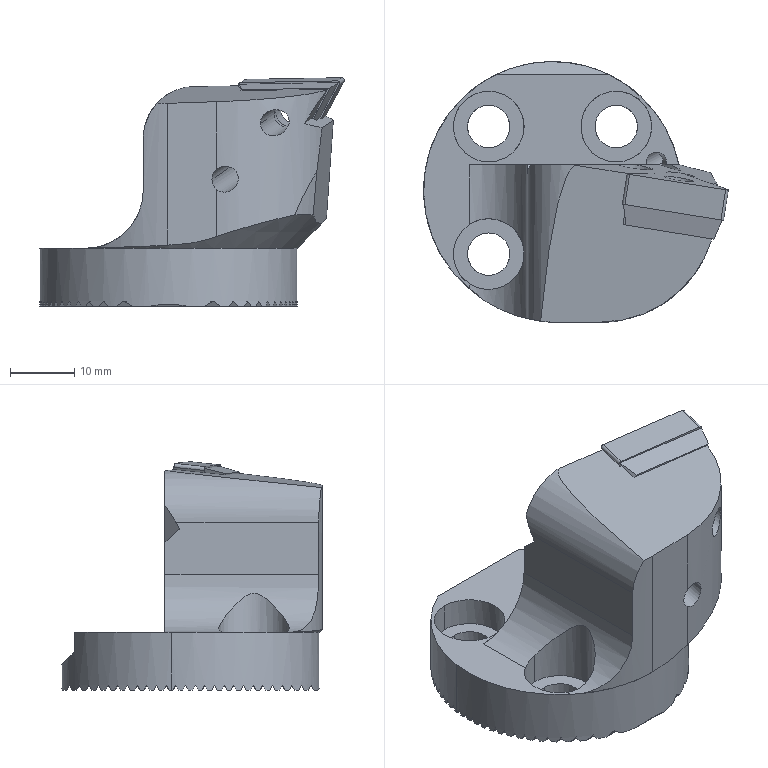NC program | Mastercam | posted with a generic post
Lines 243 to 895 of 11065:
(12 FEMR |TOOL - 4|DIA. OFF. - 4|LEN. - 4|TOOL DIA. - 12.)
N536 T4 M6
N538 G0 G54 G90 X36.247 Y-2.28 C0. B0. S3500 M3
N540 G43 H4 Z84.239 M8
N542 Z36.239
N544 G1 Z8.489 F2000.
N546 X34.611 Y-1.757 Z8.338 F2500.
N548 G3 X33.789 Y-1.629 Z8.265 I-.822 J-2.572
N550 X33.497 Y-1.645 Z8.239 J-2.7
N552 G1 X32.902 Y-1.71
N554 X32.852 Y-1.819
N556 G3 X32.449 Y-4.11 I31.093 J-6.656
N558 G2 X30.953 Y-10.357 I-38.311 J5.87
N560 X-.001 Y-32.641 I-30.954 J10.357
N562 X-6.571 Y-31.973 J32.641
N564 X-17.793 Y-27.363 I6.574 J31.969
N566 G1 X-18.064 Y-27.656
N568 X-18.335 Y-27.949
N570 G3 X-18.91 Y-28.91 Z8.314 I1.979 J-1.836
N572 G1 X-19.466 Y-30.534 Z8.428
N574 G3 X-19.604 Y-31.36 Z8.483 I2.412 J-.826
N576 X-19.603 Y-31.444 Z8.489 I2.55
N578 X-17.107 Y-33.91 I2.549 J.084
N580 G1 X-.868 Y-34.244 F9500.
N582 G3 X-.127 Y-34.252 I.741 J35.984
N584 X31.322 Y-15.762 J35.992
N586 G1 X37.454 Y-4.742
N588 G3 X37.66 Y-3.946 I-1.431 J.796
N590 X37.04 Y-2.662 I-1.637
N592 X36.521 Y-2.386 Z8.45 I-1.017 J-1.284 F2500.
N594 G1 X36.203 Y-2.284 Z8.428
N596 X34.567 Y-1.762 Z8.314
N598 G3 X33.746 Y-1.634 Z8.259 I-.821 J-2.572
N600 X33.453 Y-1.65 Z8.239 J-2.7
N602 X32.834 Y-1.719 I1.106 J-12.744
N604 X32.564 Y-2.575 I4.195 J-1.792
N606 X31.942 Y-5.531 I77.744 J-17.907
N608 G2 X29.792 Y-12.57 I-36.645 J7.343
N610 X-.001 Y-32.335 I-29.793 J12.572
N612 X-9.419 Y-30.933 J32.337
N614 X-16.595 Y-27.761 I9.618 J31.47
N616 G3 X-17.657 Y-27.216 I-13.044 J-24.096
N618 G1 X-17.928 Y-27.509
N620 X-18.199 Y-27.802
N622 G3 X-18.774 Y-28.763 Z8.314 I1.98 J-1.836
N624 G1 X-19.33 Y-30.388 Z8.428
N626 G3 X-19.456 Y-31.148 Z8.479 I2.222 J-.76
N628 X-19.452 Y-31.298 Z8.489 I2.348
N630 X-17.171 Y-33.497 I2.344 J.15 F9500.
N632 G1 X-1.185 Y-33.928
N634 G3 X-.211 Y-33.941 I.974 J36.066
N636 X31.06 Y-15.859 J36.079
N638 G1 X37.416 Y-4.815
N640 G3 X37.638 Y-3.986 I-1.44 J.829
N642 X36.975 Y-2.659 I-1.662
N644 X36.482 Y-2.404 Z8.452 I-.999 J-1.327 F2500.
N646 G1 X36.132 Y-2.292 Z8.428
N648 X34.496 Y-1.77 Z8.314
N650 G3 X33.675 Y-1.642 Z8.259 I-.821 J-2.572
N652 X33.382 Y-1.657 Z8.239 J-2.7
N654 X32.754 Y-1.734 I.357 J-5.533
N656 X32.437 Y-2.553 I3.723 J-1.913
N658 X31.751 Y-5.297 I42.795 J-12.162
N660 G2 X30.136 Y-10.889 I-44.787 J9.905
N662 X4.527 Y-31.708 I-30.159 J10.938
N664 X-.005 Y-32.03 I-4.532 J31.732
N666 X-15.177 Y-28.212 J32.054
N668 G3 X-16.923 Y-27.339 I-15.286 J-28.395
N670 G2 X-17.531 Y-27.082 I4.839 J12.3
N672 G1 X-17.803 Y-27.374
N674 X-18.074 Y-27.667
N676 G3 X-18.649 Y-28.628 Z8.314 I1.98 J-1.836
N678 G1 X-19.205 Y-30.253 Z8.428
N680 G3 X-19.323 Y-30.961 Z8.476 I2.068 J-.708
N682 X-19.314 Y-31.164 Z8.489 I2.186
N684 X-17.2 Y-33.146 I2.177 J.203 F9500.
N686 G1 X-1.47 Y-33.6
N688 G3 X-.415 Y-33.615 I1.055 J36.538
N690 X30.955 Y-15.827 J36.553
N692 G1 X37.424 Y-5.012
N694 G3 X37.674 Y-4.108 I-1.511 J.904
N696 X36.898 Y-2.648 I-1.761
N698 X36.449 Y-2.431 Z8.456 I-.985 J-1.46 F2500.
N700 G1 X36.045 Y-2.302 Z8.428
N702 X34.409 Y-1.779 Z8.314
N704 G3 X33.587 Y-1.651 Z8.258 I-.822 J-2.572
N706 X33.295 Y-1.667 Z8.239 J-2.7
N708 X32.661 Y-1.759 I.037 J-2.476
N710 X32.309 Y-2.542 I3.372 J-1.988
N712 X31.562 Y-5.126 I27.904 J-9.472
N714 X31.274 Y-6.27 I24.794 J-6.838
N716 G2 X27.745 Y-15.54 I-23.921 J3.801
N718 X23.679 Y-21.111 I-31.887 J18.998
N720 X-.01 Y-31.723 I-23.689 J21.135
N722 X-14.1 Y-28.426 J31.747
N724 X-15.204 Y-27.889 I61.693 J128.335
N726 G3 X-16.845 Y-27.154 I-9.003 J-17.895
N728 G2 X-17.411 Y-26.951 I3.292 J10.078
N730 G1 X-17.682 Y-27.244
N732 X-17.953 Y-27.537
N734 G3 X-18.528 Y-28.498 Z8.314 I1.979 J-1.836
N736 G1 X-19.084 Y-30.122 Z8.428
N738 G3 X-19.211 Y-30.882 Z8.479 I2.219 J-.76
N740 X-19.206 Y-31.033 Z8.489 I2.346
N742 X-16.876 Y-33.228 I2.341 J.151 F9500.
N744 G1 X-1.881 Y-33.299
N746 X-1.69
N748 G3 X21.649 Y-25.839 J40.234
N750 G1 X33.1 Y-17.685
N752 G3 X33.651 Y-16.617 I-.76 J1.068
N754 X33.49 Y-15.988 I-1.311
N756 G1 X32.1 Y-13.448
N758 G3 X31.337 Y-12.825 I-1.15 J-.629
N760 X30.95 Y-12.767 Z8.463 I-.387 J-1.252 F2500.
N762 X30.185 Y-13.013 Z8.409 J-1.31
N764 G1 X29.022 Y-13.849 Z8.314
N766 G3 X28.268 Y-14.677 Z8.239 I1.576 J-2.192
N768 G2 X25.806 Y-18.149 I-21.399 J12.567
N770 G1 X25.559 Y-18.454
N772 G2 X21.954 Y-22.481 I-33.281 J26.161
N774 X-.014 Y-31.417 I-21.968 J22.536
N776 X-13.318 Y-28.467 J31.472
N778 G3 X-16.062 Y-27.241 I-35.078 J-74.802
N780 X-17.292 Y-26.823 I-3.805 J-9.188
N782 G1 X-17.563 Y-27.116
N784 X-17.835 Y-27.409
N786 G3 X-18.409 Y-28.37 Z8.314 I1.98 J-1.835
N788 G1 X-18.966 Y-29.994 Z8.428
N790 G3 X-19.142 Y-30.899 Z8.489 I3.191 J-1.093
N792 X-19.147 Y-31.087 I3.367 J-.188 F9500.
N794 X-15.775 Y-34.459 I3.372
N796 X-15.493 Y-34.447 J3.372
N798 G1 X4.83 Y-32.738
N800 G3 X9.097 Y-31.619 I-1.075 J12.787
N802 G1 X30.901 Y-21.635
N804 G3 X32.81 Y-18.661 I-1.362 J2.974
N806 X30.922 Y-15.697 I-3.271
N808 X30.03 Y-15.499 I-.892 J-1.911
N810 X29.647 Y-15.534 J-2.109
N812 X29.044 Y-15.744 Z8.447 I.383 J-2.074 F2500.
N814 G1 X28.541 Y-16.01 Z8.409
N816 X27.275 Y-16.679 Z8.314
N818 G3 X26.415 Y-17.397 Z8.239 I1.263 J-2.387
N820 G2 X24.073 Y-19.978 I-20.092 J15.879
N822 G3 X23.248 Y-20.818 I165.576 J-163.477
N824 G2 X18.441 Y-25.058 I-27.559 J26.399
N826 X-.017 Y-31.107 I-18.458 J25.135
N828 X-12.326 Y-28.576 J31.184
N830 X-14.916 Y-27.464 I64.34 J153.474
N832 G3 X-17.175 Y-26.697 I-5.203 J-11.605
N834 G1 X-17.446 Y-26.989
N836 X-17.717 Y-27.282
N838 G3 X-18.292 Y-28.243 Z8.314 I1.979 J-1.836
N840 G1 X-18.848 Y-29.868 Z8.428
N842 G3 X-19.014 Y-30.774 Z8.489 I2.946 J-1.009
N844 X-19.016 Y-30.877 I3.112 J-.103 F9500.
N846 X-15.902 Y-33.991 I3.114
N848 X-15.672 Y-33.982 J3.114
N850 G1 X4.05 Y-32.522
N852 G3 X9.513 Y-31.076 I-1.136 J15.335
N854 G1 X29.143 Y-21.749
N856 G3 X30.324 Y-19.88 I-.888 J1.869
N858 X28.255 Y-17.811 I-2.069
N860 X28.155 Y-17.813 J-2.069
N862 X27.485 Y-17.959 Z8.443 I.1 J-2.067 F2500.
N864 G1 X27.002 Y-18.152 Z8.409
N866 X25.673 Y-18.685 Z8.314
N868 G3 X24.742 Y-19.308 Z8.239 I1.004 J-2.506
N870 G2 X22.509 Y-21.34 I-18.591 J18.186
N872 G3 X21.34 Y-22.355 I128.103 J-148.817
N874 G2 X16.202 Y-26.2 I-25.32 J28.475
N876 X-.016 Y-30.8 I-16.218 J26.29
N878 X-11.322 Y-28.656 J30.89
N880 X-14.701 Y-27.292 I50.742 J130.517
N882 G3 X-16.603 Y-26.668 I-4.928 J-11.813
N884 X-16.843 Y-26.644 I-.24 J-1.176
N886 X-17.167 Y-26.688 J-1.2
N888 G1 X-17.438 Y-26.981
N890 G3 X-18.013 Y-27.942 Z8.314 I1.98 J-1.836
N892 G1 X-18.569 Y-29.567 Z8.428
N894 G3 X-18.768 Y-30.468 Z8.489 I3.887 J-1.33
N896 X-18.79 Y-30.897 I4.086 J-.429 F9500.
N898 X-14.682 Y-35.005 I4.108
N900 X-14.026 Y-34.953 J4.108
N902 G1 X24.154 Y-28.77
N904 G3 X29.084 Y-22.977 I-.938 J5.793
N906 X29.054 Y-22.372 I-5.868
N908 X26.772 Y-19.805 I-2.925 J-.303
N910 X26.129 Y-19.734 Z8.446 I-.643 J-2.87 F2500.
N912 X25.57 Y-19.788 Z8.409 J-2.941
N914 G1 X24.2 Y-20.203 Z8.314
N916 G3 X23.219 Y-20.743 Z8.239 I.783 J-2.584
N918 G2 X20.901 Y-22.524 I-17.704 J20.642
N920 X17.509 Y-25.008 I-50.404 J65.266
N922 X5.266 Y-30.032 I-17.7 J25.706
N924 X-.013 Y-30.489 I-5.279 J30.25
N926 X-10.713 Y-28.565 J30.707
N928 X-14.149 Y-27.246 I39.443 J107.959
N930 G3 X-16.048 Y-26.631 I-5.62 J-14.095
N932 X-16.538 Y-26.552 I-1.135 J-5.491
N934 X-16.719 Y-26.538 I-.181 J-1.186
N936 X-17.078 Y-26.593 J-1.2
N938 G1 X-17.35 Y-26.886
N940 G3 X-17.924 Y-27.847 Z8.314 I1.98 J-1.836
N942 G1 X-18.481 Y-29.471 Z8.428
N944 G3 X-18.642 Y-30.378 Z8.489 I2.838 J-.972
N946 X-18.643 Y-30.443 I2.999 J-.065 F9500.
N948 X-15.643 Y-33.443 I3.
N950 X-15.335 Y-33.427 J3.
N952 G1 X24.409 Y-29.318
N954 G3 X28.253 Y-25.056 I-.441 J4.262
N956 X25.764 Y-21.165 I-4.285
N958 X25.269 Y-21.035 I-.618 J-1.338
N960 X25.146 Y-21.03 Z8.481 I-.123 J-1.468 F2500.
N962 X24.837 Y-21.062 Z8.46 J-1.473
N964 G1 X24.078 Y-21.225 Z8.409
N966 X22.678 Y-21.526 Z8.314
N968 G3 X21.656 Y-21.983 Z8.239 I.567 J-2.64
N970 G2 X19.564 Y-23.355 I-16.142 J22.335
N972 G3 X17.62 Y-24.631 I65.54 J-101.91
N974 G2 X11.496 Y-27.911 I-19.964 J29.922
N976 X-.017 Y-30.181 I-11.513 J28.063
N978 X-9.597 Y-28.629 J30.333
N980 X-13.542 Y-27.21 I31.389 J93.479
N982 G3 X-15.801 Y-26.517 I-5.492 J-13.885
N984 X-16.413 Y-26.434 I-1.128 J-6.029
N986 X-16.546 Y-26.427 I-.133 J-1.193
N988 X-17.012 Y-26.521 J-1.2
N990 G1 X-16.52 Y-27.357 Z8.303
N992 G3 X-14.808 Y-29.563 Z8.489 I9.389 J5.52
N994 X-7.131 Y-32.729 I7.677 J7.726 F9500.
N996 X-5.748 Y-32.641 J10.892
N998 G1 X22.916 Y-28.972
N1000 G3 X26.177 Y-25.267 I-.474 J3.705
N1002 X25.894 Y-23.837 I-3.735
N1004 X24.004 Y-22.27 I-2.428 J-1.006
N1006 X23.466 Y-22.214 Z8.453 I-.538 J-2.573 F2500.
N1008 X23.085 Y-22.242 Z8.428 J-2.629
N1010 G1 X22.803 Y-22.284 Z8.409
N1012 X21.386 Y-22.491 Z8.314
N1014 G3 X20.335 Y-22.879 Z8.239 I.391 J-2.671
N1016 G2 X18.162 Y-24.109 I-15.035 J24.043
N1018 G3 X15.793 Y-25.472 I67.843 J-120.67
N1020 G2 X8.976 Y-28.494 I-17.237 J29.68
N1022 X-.021 Y-29.871 I-8.997 J28.71
N1024 X-8.974 Y-28.508 J30.087
N1026 X-12.977 Y-27.146 I25.503 J81.551
N1028 G3 X-15.351 Y-26.435 I-6.444 J-17.201
N1030 X-16.329 Y-26.311 I-1.21 J-5.612
N1032 X-16.422 Y-26.307 I-.093 J-1.196
N1034 X-16.909 Y-26.411 J-1.2
N1036 G1 X-17.181 Y-26.703
N1038 G3 X-17.755 Y-27.665 Z8.314 I1.98 J-1.836
N1040 G1 X-18.312 Y-29.289 Z8.428
N1042 G3 X-18.458 Y-30.164 Z8.487 I2.555 J-.875
N1044 G1 X-18.457 Y-30.198 Z8.489
N1046 G3 X-15.757 Y-32.864 I2.7 J.034 F9500.
N1048 X-15.455 Y-32.847 J2.7
N1050 G1 X21.975 Y-28.63
N1052 G3 X24.373 Y-25.947 I-.302 J2.683
N1054 X22.647 Y-23.428 I-2.7
N1056 X21.673 Y-23.246 Z8.423 I-.974 J-2.519 F2500.
N1058 X21.46 Y-23.255 Z8.409 J-2.701
N1060 G1 X20.032 Y-23.368 Z8.314
N1062 G3 X18.958 Y-23.686 Z8.239 I.213 J-2.692
N1064 G2 X16.768 Y-24.747 I-14.642 J27.432
N1066 G3 X14.332 Y-25.978 I58.36 J-118.549
N1068 G2 X7.364 Y-28.632 I-15.607 J30.501
N1070 X-.021 Y-29.559 I-7.385 J28.954
N1072 X-8.293 Y-28.391 J29.881
N1074 X-12.361 Y-27.089 I20.517 J71.123
N1076 G3 X-14.854 Y-26.354 I-7.88 J-22.139
N1078 X-16.206 Y-26.186 I-1.459 J-6.206
N1080 X-16.254 Y-26.185 I-.048 J-1.199
N1082 X-16.844 Y-26.34 J-1.2
N1084 G1 X-16.298 Y-27.118 Z8.302
N1086 G3 X-14.407 Y-29.2 Z8.489 I9.223 J6.477
N1088 X-7.075 Y-31.911 I7.332 J8.559 F9500.
N1090 X-6.787 Y-31.908 J11.27
N1092 G1 X19.183 Y-31.243
N1094 G3 X22.95 Y-27.379 I-.098 J3.864
N1096 X21.818 Y-24.646 I-3.865
N1098 X21.296 Y-24.277 I-1.327 J-1.327
N1100 X20.491 Y-24.096 Z8.434 I-.805 J-1.696 F2500.
N1102 G1 X20.462 Z8.432
N1104 X20.113 Y-24.101 Z8.409
N1106 X18.682 Y-24.124 Z8.314
N1108 G3 X17.59 Y-24.373 Z8.239 I.041 J-2.699
N1110 G2 X15.621 Y-25.186 I-12.347 J27.083
N1112 G3 X12.817 Y-26.417 I41.26 J-97.851
N1114 G2 X5.702 Y-28.691 I-13.829 J30.998
N1116 X-.017 Y-29.246 I-5.719 J29.18
N1118 X-7.632 Y-28.255 J29.735
N1120 X-12.123 Y-26.899 I18.547 J69.574
N1122 G3 X-14.888 Y-26.162 I-6.979 J-20.611
N1124 X-15.985 Y-26.059 I-1.097 J-5.808
N1126 X-16.115 Y-26.06 J-5.911
N1128 G1 X-16.119
N1130 G3 X-16.752 Y-26.241 J-1.2
N1132 G1 X-16.187 Y-26.998 Z8.302
N1134 G3 X-14.23 Y-29.025 Z8.489 I8.94 J6.669
N1136 X-7.467 Y-31.48 I6.983 J8.696 F9500.
N1138 G1 X17.936 Y-31.98
N1140 G3 X18.012 Y-31.981 I.076 J3.825
N1142 X21.838 Y-28.155 J3.826
N1144 X20.766 Y-25.5 I-3.826
N1146 X20.134 Y-25.024 I-1.81 J-1.745
N1148 X19.047 Y-24.732 Z8.414 I-1.178 J-2.221 F2500.
N1150 G1 X18.973 Y-24.73 Z8.409
N1152 X17.542 Y-24.677 Z8.314
N1154 G3 X17.443 Y-24.675 Z8.307 I-.099 J-2.699
N1156 X16.438 Y-24.869 Z8.239 J-2.701
N1158 G2 X14.295 Y-25.623 I-11.342 J28.834
N1160 G3 X11.423 Y-26.717 I38.567 J-105.517
N1162 G2 X4.672 Y-28.562 I-12.378 J32.029
N1164 X-.011 Y-28.933 I-4.683 J29.332
N1166 X-7.236 Y-28.041 J29.703
N1168 X-11.741 Y-26.752 I17.876 J70.99
N1170 G3 X-14.572 Y-26.031 I-7.312 J-22.781
N1172 X-15.724 Y-25.925 I-1.152 J-6.209
N1174 X-16.051 Y-25.934 J-6.315
N1176 X-16.612 Y-26.09 I.033 J-1.199
N1178 G1 X-16.883 Y-26.383
N1180 G3 X-17.604 Y-28.219 Z8.373 I1.979 J-1.836
N1182 X-17.056 Y-29.85 Z8.489 I2.7
N1184 X-14.904 Y-30.919 I2.152 J1.631 F9500.
N1186 G1 X-14.877
N1188 X16.018 Y-30.61
N1190 G3 X18.691 Y-27.91 I-.027 J2.7
N1192 X18.363 Y-26.62 I-2.7
N1194 X15.991 Y-25.21 Z8.297 I-2.372 J-1.29 F2500.
N1196 X15.132 Y-25.35 Z8.239 J-2.7
N1198 G2 X13.153 Y-25.927 I-8.764 J26.388
N1200 G3 X10.301 Y-26.856 I21.115 J-69.679
N1202 G2 X3.499 Y-28.415 I-11.139 J32.965
N1204 X.006 Y-28.62 I-3.493 J29.682
N1206 X-6.976 Y-27.793 J29.887
N1208 X-11.476 Y-26.567 I18.533 J76.873
N1210 G3 X-14.329 Y-25.883 I-7.14 J-23.509
N1212 X-15.475 Y-25.785 I-1.146 J-6.63
N1214 X-15.949 Y-25.802 J-6.728
N1216 X-16.505 Y-25.975 I.069 J-1.198
N1218 G1 X-16.777 Y-26.268
N1220 G3 X-17.497 Y-28.104 Z8.373 I1.98 J-1.836
N1222 X-16.949 Y-29.735 Z8.489 I2.7
N1224 X-14.815 Y-30.804 I2.152 J1.631 F9500.
N1226 G1 X14.7 Y-31.001
N1228 X14.718
N1230 G3 X17.418 Y-28.301 J2.7
N1232 X17.151 Y-27.131 I-2.7
N1234 X14.718 Y-25.601 Z8.288 I-2.433 J-1.17 F2500.
N1236 X13.988 Y-25.702 Z8.239 J-2.7
N1238 G2 X11.979 Y-26.18 I-7.83 J28.463
N1240 G3 X9.121 Y-26.963 I14.784 J-59.541
N1242 G2 X2.746 Y-28.186 I-9.822 J33.978
N1244 X.037 Y-28.308 I-2.709 J30.133
N1246 X-6.759 Y-27.534 J30.255
N1248 X-11.247 Y-26.369 I19.544 J84.516
N1250 G3 X-14.117 Y-25.726 I-6.849 J-23.85
N1252 X-15.192 Y-25.635 I-1.075 J-6.29
N1254 X-15.843 Y-25.669 J-6.381
N1256 X-16.407 Y-25.869 I.107 J-1.195
N1258 G1 X-15.825 Y-26.608 Z8.301
N1260 G3 X-14.075 Y-27.613 Z8.439 I2.122 J1.67
N1262 G1 X-13.321 Y-27.718 Z8.489
N1264 X14.45 Y-31.582 F9500.
N1266 G3 X14.822 Y-31.608 I.372 J2.674
N1268 X17.522 Y-28.908 J2.7
N1270 X16.439 Y-26.746 I-2.7
N1272 X15.343 Y-26.259 Z8.409 I-1.617 J-2.162 F2500.
N1274 G1 X13.938 Y-25.983 Z8.314
N1276 G3 X13.417 Y-25.932 Z8.279 I-.521 J-2.649
N1278 X12.818 Y-25.999 Z8.239 J-2.7
N1280 G2 X10.8 Y-26.375 I-6.067 J27.005
N1282 G3 X7.925 Y-27.023 I11.157 J-56.153
N1284 G2 X1.505 Y-27.965 I-8.327 J34.394
N1286 X.12 Y-27.996 I-1.385 J31.308
N1288 X-6.98 Y-27.181 J31.339
N1290 X-11.018 Y-26.171 I26.485 J114.404
N1292 G3 X-13.908 Y-25.565 I-6.625 J-24.424
N1294 X-14.929 Y-25.485 I-1.021 J-6.459
N1296 X-15.733 Y-25.535 J-6.539
N1298 X-16.31 Y-25.764 I.14 J-1.191
N1300 G1 X-15.706 Y-26.479 Z8.301
N1302 G3 X-14.085 Y-27.401 Z8.427 I2.063 J1.742
N1304 G1 X-13.167 Y-27.553 Z8.489
N1306 X13.06 Y-31.904 F9500.
N1308 G3 X13.501 Y-31.94 I.441 J2.663
N1310 X16.2 Y-29.241 J2.699
N1312 X15.224 Y-27.162 I-2.699
N1314 X14.153 Y-26.621 Z8.409 I-1.723 J-2.079 F2500.
N1316 G1 X12.763 Y-26.275 Z8.314
N1318 G3 X12.112 Y-26.195 Z8.27 I-.651 J-2.62
N1320 X11.644 Y-26.236 Z8.239 J-2.7
N1322 G2 X9.607 Y-26.513 I-4.941 J28.719
N1324 G3 X6.697 Y-27.036 I9.045 J-58.635
N1326 G2 X.237 Y-27.691 I-6.78 J34.694
N1328 X-7.211 Y-26.83 I.07 J33.264
N1330 X-11.167 Y-25.88 I37.185 J163.526
N1332 G3 X-13.985 Y-25.37 I-5.228 J-20.837
N1334 X-14.694 Y-25.33 I-.709 J-6.257
N1336 X-15.652 Y-25.404 J-6.297
N1338 X-16.166 Y-25.609 I.177 J-1.186
N1340 G1 X-16.438 Y-25.902
N1342 G3 X-17.158 Y-27.738 Z8.373 I1.98 J-1.836
N1344 X-16.61 Y-29.369 Z8.489 I2.7
N1346 X-14.602 Y-30.434 I2.152 J1.631 F9500.
N1348 G1 X10.651 Y-31.789
N1350 G3 X10.795 Y-31.793 I.144 J2.696
N1352 X13.495 Y-29.093 J2.7
N1354 X13.376 Y-28.298 I-2.7
N1356 X10.795 Y-26.392 Z8.261 I-2.581 J-.795 F2500.
N1358 X10.46 Y-26.414 Z8.239 J-2.701
N1360 G2 X8.403 Y-26.593 I-3.799 J31.699
N1362 G3 X5.442 Y-26.997 I7.694 J-67.42
N1364 G2 X.258 Y-27.382 I-5.184 J34.681
N1366 X-1.518 Y-27.338 J35.066
N1368 X-7.868 Y-26.392 I2.439 J38.179
N1370 X-10.609 Y-25.758 I56.647 J251.007
N1372 G3 X-13.525 Y-25.229 I-6.077 J-25.191
N1374 X-14.431 Y-25.174 I-.906 J-7.399
N1376 X-15.328 Y-25.228 J-7.454
N1378 X-16.088 Y-25.525 I.09 J-1.349
N1380 X-14.723 Y-26.321 Z8.345 I1.982 J1.833
N1382 G1 X-12.614 Y-26.816 Z8.489
N1384 X8.854 Y-31.854 F9500.
N1386 G3 X9.471 Y-31.925 I.617 J2.629
N1388 X12.171 Y-29.225 J2.7
N1390 X12.087 Y-28.559 I-2.7
N1392 X9.471 Y-26.526 Z8.252 I-2.616 J-.666 F2500.
N1394 X9.269 Y-26.533 Z8.239 J-2.699
N1396 G2 X7.259 Y-26.612 I-2.384 J34.808
N1398 G3 X4.272 Y-26.892 I5.178 J-71.278
N1400 G2 X.517 Y-27.092 I-3.755 J35.107
N1402 X-6.728 Y-26.341 J35.307
N1404 X-10.688 Y-25.49 I29.702 J147.753
N1406 G3 X-13.551 Y-25.038 I-4.989 J-22.313
N1408 X-14.19 Y-25.008 I-.639 J-6.746
N1410 X-15.277 Y-25.096 J-6.776
N1412 X-15.936 Y-25.362 I.152 J-1.326
N1414 G1 X-16.208 Y-25.654
N1416 G3 X-16.928 Y-27.49 Z8.373 I1.98 J-1.836
N1418 X-16.38 Y-29.121 Z8.489 I2.7
N1420 X-14.444 Y-30.182 I2.152 J1.631 F9500.
N1422 G1 X7.988 Y-31.981
N1424 G3 X8.204 Y-31.99 I.216 J2.691
N1426 X10.904 Y-29.29 J2.7
N1428 X10.849 Y-28.749 I-2.7
N1430 X8.204 Y-26.59 Z8.244 I-2.645 J-.541 F2500.
N1432 X8.13 Y-26.591 Z8.239 J-2.7
N1434 G2 X6.235 Y-26.608 I-1.895 J103.417
N1436 X5.667 Y-26.607 J103.434
N1438 G3 X2.53 Y-26.766 I4.492 J-119.683
N1440 G2 X.793 Y-26.806 I-1.737 J37.987
N1442 X-6.996 Y-25.999 J38.027
N1444 X-10.52 Y-25.277 I44.26 J224.921
N1446 G3 X-13.39 Y-24.863 I-4.686 J-22.33
N1448 X-13.947 Y-24.841 I-.557 J-6.891
N1450 X-15.137 Y-24.944 J-6.913
N1452 X-15.817 Y-25.233 I.19 J-1.392
N1454 G1 X-16.089 Y-25.526
N1456 G3 X-16.809 Y-27.362 Z8.373 I1.98 J-1.836
N1458 X-16.261 Y-28.992 Z8.489 I2.7
N1460 X-14.361 Y-30.05 I2.152 J1.63 F9500.
N1462 G1 X6.319 Y-31.988
N1464 G3 X6.571 Y-32. I.252 J2.688
N1466 X9.271 Y-29.3 J2.7
N1468 X9.23 Y-28.831 I-2.7
N1470 X6.571 Y-26.6 Z8.239 I-2.659 J-.469 F2500.
N1472 G1 X5.972
N1474 G2 X4.177 Y-26.602 I-1.795 J842.669
N1476 X-.46 Y-26.589 J842.671
N1478 X-7.652 Y-25.592 I4.109 J56.073
N1480 X-9.227 Y-25.28 I71.544 J365.141
N1482 G3 X-12.639 Y-24.729 I-7.241 J-33.993
N1484 X-13.624 Y-24.674 I-.985 J-8.754
N1486 X-14.825 Y-24.756 J-8.809
N1488 X-15.572 Y-25.013 I.26 J-1.971
N1490 X-15.775 Y-25.187 I.677 J-.99
N1492 X-16.495 Y-27.023 Z8.373 I1.98 J-1.836
N1494 X-15.947 Y-28.654 Z8.489 I2.7
N1496 X-14.266 Y-29.682 I2.152 J1.631 F9500.
N1498 G1 X-1.796 Y-31.893
N1500 G3 X-1.325 Y-31.934 I.471 J2.659
N1502 X1.375 Y-29.234 J2.7
N1504 X1.364 Y-28.986 I-2.7
N1506 X-1.102 Y-26.543 Z8.239 I-2.689 J-.248 F2500.
N1508 G2 X-5.96 Y-25.717 I2.47 J29.206
N1510 G3 X-11.068 Y-24.713 I-19.815 J-87.349
N1512 X-13.611 Y-24.503 I-2.543 J-15.302
N1514 X-13.724 Y-24.504 J-15.512
N1516 X-15.105 Y-24.705 I.007 J-4.883
N1518 X-15.636 Y-25.037 I.349 J-1.148
N1520 X-16.356 Y-26.873 Z8.373 I1.98 J-1.836
N1522 X-15.808 Y-28.504 Z8.489 I2.7
N1524 X-14.214 Y-29.515 I2.152 J1.631 F9500.
N1526 G1 X-6.192 Y-31.21
N1528 G3 X-5.633 Y-31.268 I.559 J2.642
N1530 X-2.937 Y-28.702 J2.7
N1532 X-2.934 Y-28.568 Z8.48 I-2.696 J.134 F2500.
N1534 X-5.033 Y-25.936 Z8.239 I-2.699
N1536 G2 X-7.674 Y-25.206 I7.4 J31.932
N1538 G3 X-12.476 Y-24.352 I-7.026 J-25.579
N1540 X-13.155 Y-24.324 I-.679 J-8.281
N1542 X-14.602 Y-24.451 J-8.309
N1544 X-15.344 Y-24.748 I.312 J-1.858
N1546 X-15.493 Y-24.884 I.731 J-.952
N1548 X-16.213 Y-26.72 Z8.373 I1.98 J-1.836
N1550 X-15.665 Y-28.35 Z8.489 I2.7
N1552 X-14.106 Y-29.354 I2.152 J1.63 F9500.
N1554 G1 X-8.192 Y-30.685
N1556 G3 X-7.599 Y-30.751 I.593 J2.634
N1558 X-4.917 Y-28.363 J2.7
N1560 X-4.899 Y-28.051 Z8.468 I-2.682 J.312 F2500.
N1562 X-6.826 Y-25.464 Z8.239 I-2.7
N1564 G2 X-8.759 Y-24.82 I11.159 J36.732
N1566 G3 X-13.226 Y-24.16 I-4.467 J-14.784
N1568 X-13.327 Y-24.161 J-15.444
N1570 X-14.885 Y-24.418 I.034 J-5.049
N1572 X-15.348 Y-24.727 I.417 J-1.125
N1574 G1 X-15.62 Y-25.02
N1576 G3 X-16.34 Y-26.856 Z8.373 I1.98 J-1.836
N1578 X-15.792 Y-28.487 Z8.489 I2.7
N1580 X-14.081 Y-29.52 I2.152 J1.631 F9500.
N1582 G1 X-9.288 Y-30.313
N1584 G3 X-8.848 Y-30.349 I.44 J2.664
N1586 X-6.181 Y-28.075 J2.7
N1588 X-6.147 Y-27.649 Z8.461 I-2.667 J.426 F2500.
N1590 X-7.966 Y-25.097 Z8.239 I-2.701
N1592 G2 X-9.46 Y-24.54 I9.053 J26.559
N1594 G3 X-12.888 Y-23.999 I-3.428 J-10.595
N1596 X-13.583 Y-24.021 J-11.136
N1598 X-14.739 Y-24.26 I.298 J-4.352
N1600 X-15.202 Y-24.569 I.417 J-1.125
N1602 G1 X-15.473 Y-24.862
N1604 G3 X-16.193 Y-26.698 Z8.373 I1.98 J-1.836
N1606 X-15.645 Y-28.329 Z8.489 I2.7
N1608 X-13.948 Y-29.359 I2.152 J1.631 F9500.
N1610 G1 X-10.125 Y-30.013
N1612 G3 X-9.67 Y-30.052 I.455 J2.662
N1614 X-7.017 Y-27.853 J2.701
N1616 X-6.97 Y-27.351 Z8.456 I-2.653 J.502 F2500.
N1618 X-8.716 Y-24.826 Z8.239 I-2.7
N1620 G2 X-10.01 Y-24.3 I9.931 J26.287
N1622 G3 X-12.784 Y-23.845 I-2.774 J-8.221
N1624 X-13.764 Y-23.9 J-8.676
N1626 X-14.613 Y-24.11 I.419 J-3.513
N1628 X-15.055 Y-24.412 I.437 J-1.118
N1630 G1 X-15.327 Y-24.704
N1632 G3 X-16.047 Y-26.54 Z8.373 I1.98 J-1.836
N1634 X-15.499 Y-28.171 Z8.489 I2.7
N1636 X-13.803 Y-29.201 I2.152 J1.631 F9500.
N1638 G1 X-10.94 Y-29.692
N1640 G3 X-10.484 Y-29.731 I.456 J2.661
N1642 X-7.846 Y-27.607 J2.7
N1644 X-7.784 Y-27.031 Z8.451 I-2.638 J.576 F2500.
N1646 X-9.459 Y-24.533 Z8.239 I-2.7
N1648 G2 X-10.51 Y-24.082 I22.227 J53.298
N1650 G3 X-12.756 Y-23.703 I-2.246 J-6.471
N1652 X-14.07 Y-23.831 J-6.85
N1654 X-14.788 Y-24.141 I.317 J-1.721
N1656 X-15.183 Y-24.549 I2.089 J-2.415
N1658 X-15.903 Y-26.385 Z8.373 I1.98 J-1.836
N1660 X-15.355 Y-28.016 Z8.489 I2.7
N1662 X-13.748 Y-29.029 I2.152 J1.631 F9500.
N1664 G1 X-11.433 Y-29.506
N1666 G3 X-10.888 Y-29.562 I.545 J2.644
N1668 X-8.258 Y-27.475 J2.7
N1670 X-8.188 Y-26.862 Z8.448 I-2.63 J.613 F2500.
N1672 X-9.827 Y-24.379 Z8.239 I-2.7
N1674 G2 X-10.875 Y-23.91 I10.926 J25.836
N1676 G3 X-12.794 Y-23.574 I-1.919 J-5.317
N1678 X-14.091 Y-23.725 J-5.653
N1680 X-14.774 Y-24.108 I.292 J-1.321
N1682 G1 X-15.046 Y-24.401
N1684 G3 X-15.766 Y-26.237 Z8.373 I1.98 J-1.836
N1686 X-15.218 Y-27.868 Z8.489 I2.7
N1688 X-13.722 Y-28.856 I2.152 J1.631 F9500.
N1690 G1 X-11.97 Y-29.295
N1692 G3 X-11.314 Y-29.376 I.656 J2.619
N1694 X-8.694 Y-27.329 J2.7
N1696 X-8.614 Y-26.676 Z8.445 I-2.62 J.653 F2500.
N1698 X-10.215 Y-24.209 Z8.239 I-2.7
N1700 G2 X-11.227 Y-23.741 I25.948 J57.362
N1702 G3 X-12.857 Y-23.456 I-1.63 J-4.524
N1704 X-13.92 Y-23.575 J-4.809
N1706 X-14.318 Y-23.756 I.29 J-1.164
N1708 X-14.774 Y-24.108 I1.337 J-2.204
N1710 X-15.494 Y-25.944 Z8.373 I1.98 J-1.836
N1712 X-14.946 Y-27.575 Z8.489 I2.7
N1714 X-14.019 Y-28.351 I2.152 J1.631 F9500.
N1716 G1 X-12.936 Y-28.901
N1718 G3 X-11.712 Y-29.194 I1.224 J2.406
N1720 X-9.102 Y-27.185 J2.699
N1722 X-9.012 Y-26.495 Z8.443 I-2.61 J.69 F2500.
N1724 X-10.579 Y-24.044 Z8.239 I-2.7
N1726 X-11.593 Y-23.564 I-64.721 J-135.444
N1728 X-12.911 Y-23.35 I-1.318 J-3.946
N1730 X-13.652 Y-23.417 J-4.16
N1732 X-14.112 Y-23.612 I.228 J-1.178
N1734 G1 X-14.439 Y-23.841
N1736 G3 X-14.774 Y-24.108 I.98 J-1.571
N1738 X-15.494 Y-25.944 Z8.373 I1.98 J-1.836
N1740 X-14.946 Y-27.575 Z8.489 I2.7
N1742 X-14.06 Y-28.329 I2.152 J1.631 F9500.
N1744 G1 X-13.373 Y-28.694
N1746 G3 X-12.108 Y-29.009 I1.265 J2.385
N1748 X-9.508 Y-27.036 J2.7
N1750 X-9.408 Y-26.309 Z8.44 I-2.6 J.727 F2500.
N1752 X-10.94 Y-23.874 Z8.239 I-2.7
N1754 G2 X-11.787 Y-23.45 I12.155 J25.335
N1756 G3 X-12.946 Y-23.254 I-1.159 J-3.331
N1758 X-13.408 Y-23.285 J-3.527
N1760 X-13.94 Y-23.492 I.156 J-1.19
N1762 G1 X-14.267 Y-23.721
N1764 X-14.583 Y-23.941
N1766 G3 X-15.094 Y-24.924 Z8.316 I.689 J-.983
N1768 X-14.249 Y-26.071 Z8.417 I1.2
N1770 G1 X-13.205 Y-26.394 Z8.489
N1772 X-12.418 Y-26.637 F9500.
N1774 G3 X-11.953 Y-26.707 I.465 J1.504
N1776 X-11.505 Y-26.643 J1.574
N1778 X-10.378 Y-25.133 Z8.355 I-.448 J1.51 F2500.
N1780 X-11.254 Y-23.721 Z8.239 I-1.575
N1782 X-12.053 Y-23.323 I-8.222 J-15.51
N1784 X-12.972 Y-23.171 I-.919 J-2.699
N1786 X-13.201 Y-23.18 J-2.851
N1788 X-13.801 Y-23.394 I.088 J-1.197
N1790 G1 X-14.128 Y-23.623
N1792 X-14.583 Y-23.941
N1794 G3 X-15.094 Y-24.924 Z8.315 I.689 J-.983
N1796 X-14.227 Y-26.077 Z8.418 I1.2
N1798 G1 X-13.199 Y-26.374 Z8.489
N1800 X-12.572 Y-26.555 F9500.
N1802 G3 X-12.135 Y-26.617 I.437 J1.513
N1804 X-11.698 Y-26.555 J1.575
N1806 X-10.56 Y-25.042 Z8.354 I-.437 J1.513 F2500.
N1808 X-11.427 Y-23.635 Z8.239 I-1.575
N1810 X-12.251 Y-23.218 I-8.272 J-15.343
N1812 X-12.979 Y-23.1 I-.728 J-2.184
N1814 G1 X-13.009
N1816 G3 X-13.691 Y-23.317 I.006 J-1.2
N1818 G1 X-14.018 Y-23.546
N1820 X-14.345 Y-23.775
N1822 G3 X-15.497 Y-25.987 Z8.411 I1.548 J-2.212
N1824 X-15.244 Y-27.128 Z8.489 I2.7
N1826 X-12.797 Y-28.687 I2.447 J1.141 F9500.
N1828 X-10.193 Y-26.702 J2.7
N1830 X-10.097 Y-25.987 Z8.441 I-2.604 J.715 F2500.
N1832 X-11.111 Y-23.878 Z8.28 I-2.7
N1834 G1 X-11.178 Y-23.824 Z8.275
N1836 G3 X-11.63 Y-23.532 Z8.239 I-1.686 J-2.109
N1838 X-12.382 Y-23.143 I-7.288 J-13.174